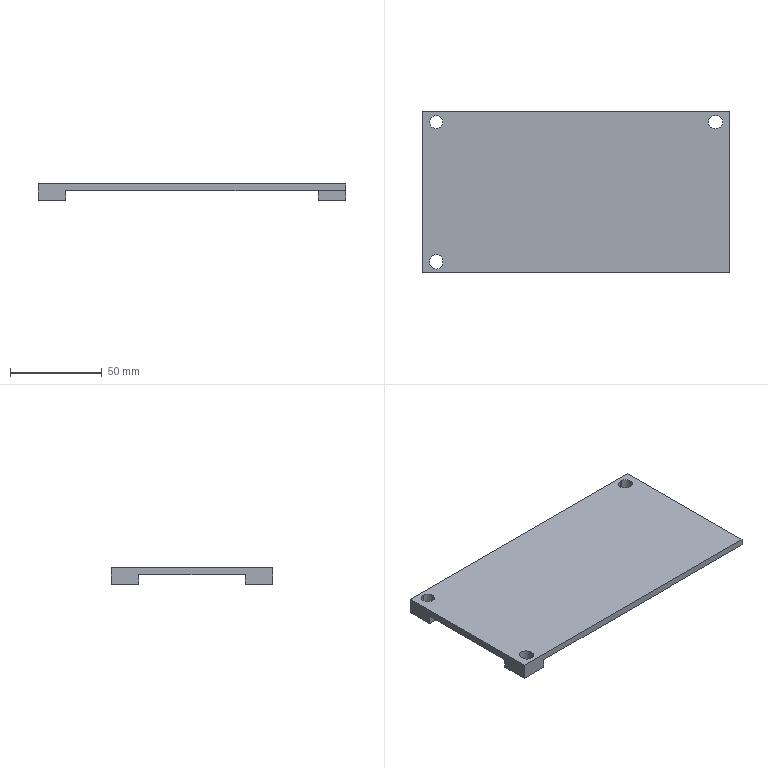NC program | NX | posted with a generic post | part box 168 x 88.2 x 8.8 mm
Lines 1 to 882 of 6992:
N10 G17 G21 G94 G90
(FLOOR_WALL , TOOL : D80)
N12 T19 M6
N14 G54
N16 G17 G0 G90 X-132. Y49.097 S5000 M3
N18 G43 Z30. H19
N20 Z3.
N22 G94 G1 Z0. F1200.
N24 X-129.
N26 X129.
N28 Y15.999
N30 X-129.
N32 Y-17.1
N34 X129.
N36 X132.
N38 Z3.
N40 G0 Z30.
N42 M5
(ADAPTIVE_MILLING , TOOL : D10)
N44 T15 M6
N46 G54
N48 G17 G0 G90 X-96.659 Y0.013 S9500 M3
N50 G43 Z30. H15
N52 Z-5.8
N54 G94 G1 Z-8.8 F1000.
N56 X-95.879 Y-0.266 F3000.
N58 X-95.09 Y-0.523
N60 G3 X-94.012 Y0.013 R1.017
N62 X-93.273 Y3.241 R9.097
N64 X-93.018 Y13.66 R133.26
N66 G1 X-93.014 Y16.36
N68 X-93.011 Y21.61
N70 Y46.135
N72 X-93.009 Y46.21
N74 X-93.003 Y46.36
N76 X-92.998 Y46.434
N78 G2 X-90.298 Y50.657 R5.929
N80 X-84.761 Y52.61 R12.858
N82 X-75.854 Y53.062 R69.734
N84 G1 X-74.504 Y53.071
N86 X-72.854 Y53.078
N88 X-70.529 Y53.083
N90 X-66.779 Y53.086
N92 X-54.779 Y53.087
N94 X85.996
N96 G2 X90.312 Y50.709 R5.649
N98 X92.436 Y45.322 R11.95
N100 X92.953 Y36.871 R57.592
N102 G1 X92.963 Y35.896
N104 X92.971 Y34.621
N106 X92.979 Y32.896
N108 X92.984 Y30.571
N110 X92.987 Y26.746
N112 X92.988 Y14.146
N114 Y-46.079
N116 X92.987 Y-46.154
N118 X92.983 Y-46.304
N120 X92.978 Y-46.379
N122 X92.972 Y-46.453
N124 G2 X90.314 Y-50.621 R5.924
N126 X84.564 Y-52.635 R12.965
N128 X75.431 Y-53.065 R74.74
N130 G1 X74.156 Y-53.073
N132 X72.431 Y-53.079
N134 X69.956 Y-53.084
N136 X65.606 Y-53.087
N138 X41.681
N140 X-35.494 Y-53.088
N142 X-36.019 Y-53.091
N144 X-37.069 Y-53.092
N146 X-37.594
N148 X-38.194 Y-53.094
N150 X-39.244
N152 X-40.144 Y-53.096
N154 X-41.344 Y-53.095
N156 X-42.019 Y-53.097
N158 X-43.219 Y-53.096
N160 X-43.819 Y-53.097
N162 X-44.944 Y-53.096
N164 X-45.319 Y-53.095
N166 X-45.994 Y-53.098
N168 X-47.269 Y-53.096
N170 X-47.944 Y-53.098
N172 X-49.144 Y-53.096
N174 X-49.969 Y-53.099
N176 X-50.719 Y-53.098
N178 X-51.769 Y-53.1
N180 X-52.444 Y-53.098
N182 X-53.569 Y-53.1
N184 X-54.169 Y-53.099
N186 X-55.294 Y-53.101
N188 X-55.669
N190 X-56.119 Y-53.1
N192 X-57.094 Y-53.101
N194 X-57.469
N196 X-57.994 Y-53.1
N198 X-59.194 Y-53.101
N200 X-59.869 Y-53.099
N202 X-61.069 Y-53.101
N204 X-61.894 Y-53.099
N206 X-63.094 Y-53.102
N208 X-63.619 Y-53.1
N210 X-65.194 Y-53.102
N212 X-65.719 Y-53.103
N214 X-66.244 Y-53.101
N216 X-67.444 Y-53.102
N218 X-68.344 Y-53.1
N220 X-69.244 Y-53.101
N222 X-69.994 Y-53.099
N224 X-71.119 Y-53.101
N226 X-71.869 Y-53.099
N228 X-72.769 Y-53.1
N230 X-73.519 Y-53.099
N232 X-74.419 Y-53.101
N234 X-75.019 Y-53.099
N236 X-76.219 Y-53.101
N238 X-76.894 Y-53.099
N240 X-77.944 Y-53.1
N242 X-78.619 Y-53.098
N244 X-79.594 Y-53.1
N246 X-80.194 Y-53.099
N248 X-81.244 Y-53.101
N250 X-81.619
N252 X-82.144 Y-53.1
N254 G2 X-86.642 Y-53.049 R55.93
N256 X-90.766 Y-50.059 R6.199
N258 X-92.602 Y-44.164 R14.147
N260 X-92.973 Y-34.276 R94.705
N262 G1 X-92.98 Y-32.626
N264 X-92.984 Y-30.151
N266 X-92.987 Y-25.876
N268 X-92.988 Y-6.526
N270 Y-3.826
N272 X-92.985 Y-3.601
N274 G2 X-92.416 Y2.144 R99.297
N276 G3 X-92.035 Y14.659 R147.053
N278 G1 X-92.029 Y16.834
N280 X-92.025 Y19.984
N282 X-92.023 Y26.209
N284 X-92.022 Y43.009
N286 X-92.02 Y43.159
N288 X-92.019 Y43.234
N290 G2 X-88.333 Y49.422 R7.66
N292 X-81.987 Y51.558 R15.465
N294 X-72.781 Y52.041 R76.235
N296 G1 X-71.581 Y52.051
N298 X-70.156 Y52.06
N300 X-68.281 Y52.067
N302 X-65.731 Y52.072
N304 X-61.381 Y52.075
N306 X-45.106 Y52.076
N308 X82.919
N310 X83.069 Y52.074
N312 X83.219 Y52.07
N314 X83.369 Y52.063
N316 X83.519 Y52.053
N318 G2 X89.452 Y48.198 R7.743
N320 X91.482 Y41.892 R15.917
N322 X91.95 Y31.859 R85.406
N324 G1 X91.96 Y30.434
N326 X91.967 Y28.634
N328 X91.972 Y26.159
N330 X91.975 Y22.109
N332 X91.977 Y9.884
N334 Y-31.216
N336 G2 X91.95 Y-43.74 R466.461
N338 X88.059 Y-49.573 R7.789
N340 X81.598 Y-51.609 R16.275
N342 X72.238 Y-52.046 R85.328
N344 G1 X70.963 Y-52.056
N346 X69.388 Y-52.063
N348 X67.288 Y-52.069
N350 X64.138 Y-52.074
N352 X57.838 Y-52.076
N354 X-32.462
N356 X-33.287 Y-52.082
N358 X-34.412
N360 X-35.237 Y-52.086
N362 X-36.287 Y-52.087
N364 X-36.662
N366 X-37.337 Y-52.09
N368 X-38.312
N370 X-39.212 Y-52.093
N372 X-40.337 Y-52.092
N374 X-41.012 Y-52.094
N376 X-41.912 Y-52.093
N378 X-42.362 Y-52.092
N380 X-43.187 Y-52.095
N382 X-44.312 Y-52.093
N384 X-44.987 Y-52.095
N386 X-46.187 Y-52.094
N388 X-46.562
N390 X-47.162 Y-52.096
N392 X-48.362 Y-52.095
N394 X-49.112 Y-52.097
N396 X-50.162 Y-52.096
N398 X-50.762 Y-52.098
N400 X-52.037 Y-52.097
N402 X-52.637 Y-52.099
N404 X-53.687 Y-52.098
N406 X-54.512 Y-52.101
N408 X-55.262 Y-52.1
N410 X-56.312 Y-52.101
N412 X-57.212 Y-52.1
N414 X-58.112 Y-52.101
N416 X-58.487 Y-52.102
N418 X-59.236 Y-52.099
N420 X-60.361 Y-52.102
N422 X-61.036 Y-52.101
N424 X-62.086 Y-52.102
N426 X-62.761 Y-52.104
N428 X-63.361 Y-52.103
N430 X-64.936
N432 X-65.686 Y-52.105
N434 X-66.211 Y-52.103
N436 X-67.261 Y-52.104
N438 X-68.161 Y-52.106
N440 X-68.761 Y-52.103
N442 X-69.886 Y-52.104
N444 G2 X-83.536 Y-52.075 R830.143
N446 X-89.419 Y-48.263 R7.764
N448 X-91.483 Y-41.891 R15.898
N450 X-91.949 Y-32.008 R84.57
N452 G1 X-91.959 Y-30.658
N454 X-91.966 Y-28.933
N456 X-91.971 Y-26.608
N458 X-91.975 Y-22.933
N460 X-91.976 Y-13.933
N462 Y-6.133
N464 G2 X-91.522 Y0.9 R88.839
N466 G3 X-91.046 Y17.013 R201.872
N468 G1 X-91.04 Y19.563
N470 X-91.036 Y23.388
N472 X-91.034 Y31.413
N474 X-91.033 Y40.038
N476 X-91.031 Y40.413
N478 X-91.027 Y40.638
N480 G2 X-87.928 Y47.368 R8.693
N482 X-85.91 Y48.894 R5.21
N484 X-78.589 Y50.684 R21.893
N486 X-67.498 Y51.046 R132.801
N488 G1 X-65.623 Y51.054
N490 X-63.148 Y51.059
N492 X-59.248 Y51.063
N494 X-49.798 Y51.064
N496 X80.327 Y51.065
N498 X80.627 Y51.06
N500 G2 X87.148 Y48.12 R8.608
N502 X88.694 Y46.211 R5.049
N504 X90.561 Y38.912 R21.152
N506 X90.944 Y28.123 R122.229
N508 G1 X90.952 Y26.473
N510 X90.958 Y24.298
N512 X90.962 Y21.073
N514 X90.965 Y14.923
N516 X90.966 Y-28.202
N518 X90.969 Y-28.802
N520 G2 X90.955 Y-41.251 R725.465
N522 X88.012 Y-47.259 R8.599
N524 X86.111 Y-48.794 R5.052
N526 X78.737 Y-50.667 R21.271
N528 X67.723 Y-51.045 R126.708
N530 G1 X65.923 Y-51.053
N532 X63.523 Y-51.059
N534 X59.998 Y-51.062
N536 X52.273 Y-51.064
N538 X-29.477 Y-51.065
N540 X-30.302 Y-51.07
N542 X-31.352 Y-51.072
N544 X-31.727
N546 X-32.252 Y-51.075
N548 X-33.602 Y-51.078
N550 X-34.127
N552 X-34.802 Y-51.082
N554 X-35.552 Y-51.083
N556 X-35.927
N558 X-36.602 Y-51.086
N560 X-37.577 Y-51.087
N562 X-37.952
N564 X-38.402 Y-51.089
N566 X-39.452
N568 X-39.827
N570 X-40.427 Y-51.092
N572 X-41.477 Y-51.091
N574 X-42.227 Y-51.093
N576 X-43.502 Y-51.091
N578 X-44.177 Y-51.093
N580 X-45.302 Y-51.092
N582 X-45.677
N584 X-46.277 Y-51.094
N586 X-47.402
N588 X-48.077 Y-51.096
N590 X-49.202 Y-51.094
N592 X-50.027 Y-51.097
N594 X-51.002 Y-51.096
N596 X-51.752 Y-51.098
N598 X-52.877 Y-51.097
N600 X-53.552 Y-51.099
N602 X-54.677 Y-51.098
N604 X-55.052
N606 X-55.652 Y-51.099
N608 X-56.552
N610 X-56.927 Y-51.098
N612 X-57.677 Y-51.101
N614 X-58.502 Y-51.1
N616 X-59.402 Y-51.102
N618 X-59.777 Y-51.103
N620 X-60.527 Y-51.102
N622 X-61.652 Y-51.104
N624 X-62.327 Y-51.103
N626 X-63.227 Y-51.104
N628 X-63.977 Y-51.102
N630 X-64.652 Y-51.104
N632 X-65.102 Y-51.105
N634 X-66.227 Y-51.102
N636 X-67.127 Y-51.105
N638 X-68.102 Y-51.102
N640 X-68.927 Y-51.104
N642 X-69.827 Y-51.102
N644 X-70.952 Y-51.104
N646 X-71.777 Y-51.102
N648 X-72.677 Y-51.103
N650 X-73.652 Y-51.101
N652 X-74.777 Y-51.103
N654 X-75.452 Y-51.102
N656 X-76.577 Y-51.103
N658 X-76.952
N660 X-77.627 Y-51.101
N662 G2 X-82.046 Y-50.974 R32.659
N664 X-87.199 Y-48.081 R8.637
N666 X-88.66 Y-46.278 R5.013
N668 X-90.56 Y-38.912 R21.138
N670 X-90.947 Y-27.447 R128.239
N672 G1 X-90.955 Y-25.572
N674 X-90.96 Y-23.097
N676 X-90.964 Y-19.197
N678 X-90.965 Y-9.447
N680 Y-7.872
N682 X-90.96 Y-7.197
N684 G2 X-90.373 Y3.135 R256.242
N686 G3 X-90.05 Y22.18 R382.724
N688 G2 X-90.009 Y39.054 R953.587
N690 X-89.166 Y42.842 R11.59
N692 X-88.948 Y45.497 R12.88
N694 X-87.915 Y47.385 R5.352
N696 G1 X-87.759 Y47.591
N698 X-87.586 Y47.784
N700 X-86.63 Y48.518
N702 X-86.511 Y48.587
N704 G2 X-83.515 Y49.254 R6.135
N706 X-66.215 Y50.03 R172.99
N708 G1 X-64.415 Y50.039
N710 X-62.09 Y50.045
N712 X-58.79 Y50.05
N714 X-52.94 Y50.052
N716 X10.735 Y50.053
N718 X78.01
N720 G2 X82.636 Y49.258 R12.734
N722 X85.397 Y49.048 R12.239
N724 X87.166 Y48.107 R5.201
N726 G1 X86.847 Y48.358
N728 X86.511 Y48.587
N730 G3 X83.965 Y49.25 R6.124
N732 G1 X82.711
N734 G3 X67.864 Y49.446 R300.003
N736 G1 X-61.661 Y49.447
N738 X-61.961 Y49.445
N740 X-62.111
N742 X-62.636 Y49.442
N744 X-62.786
N746 G3 X-74.872 Y49.25 R373.405
N748 G1 X-83.647
N750 X82.403
N752 G2 X85.397 Y49.048 R12.741
N754 X88.487 Y46.611 R5.458
N756 X89.15 Y43.69 R6.026
N758 X89.94 Y24.29 R189.119
N760 G1 X89.947 Y21.89
N762 X89.951 Y18.44
N764 X89.953 Y11.915
N766 X89.954 Y-25.21
N768 X89.958 Y-25.81
N770 X89.96 Y-26.935
N772 G2 X89.941 Y-39.309 R466.914
N774 X89.165 Y-42.732 R11.596
N776 X88.948 Y-45.497 R13.211
N778 X88.007 Y-47.266 R5.201
N780 G1 X88.258 Y-46.947
N782 X88.487 Y-46.611
N784 G3 X89.15 Y-44.065 R6.124
N786 G1 Y-42.853
N788 G3 X89.358 Y-28.833 R232.088
N790 G1 X89.354 Y-26.883
N792 X89.353 Y-25.308
N794 X89.352 Y-24.483
N796 X89.355 Y-22.683
N798 X89.353 Y-20.658
N800 Y-20.208
N802 X89.355 Y-18.483
N804 X89.354 Y-16.308
N806 X89.353 Y-15.708
N808 Y-14.883
N810 X89.354 Y-13.008
N812 X89.355 Y-12.408
N814 X89.353 Y-10.158
N816 Y-9.783
N818 X89.354 Y-7.308
N820 X89.355 Y-6.858
N822 X89.353 Y-4.608
N824 Y-4.233
N826 X89.354 Y-2.208
N828 X89.355 Y-1.833
N830 X89.353 Y0.192
N832 Y0.642
N834 X89.355 Y2.367
N836 X89.354 Y3.942
N838 X89.352 Y4.617
N840 X89.353 Y5.142
N842 X89.354 Y7.017
N844 X89.355 Y7.617
N846 X89.353 Y9.867
N848 X89.352 Y10.392
N850 X89.354 Y12.192
N852 X89.352 Y14.217
N854 X89.351 Y14.742
N856 X89.353 Y16.542
N858 X89.352 Y17.067
N860 Y17.292
N862 X89.351 Y17.592
N864 X89.352 Y17.817
N866 X89.35 Y18.492
N868 X89.351 Y18.717
N870 X89.349 Y19.092
N872 Y19.242
N874 X89.348 Y19.542
N876 X89.349 Y19.692
N878 X89.347 Y20.142
N880 Y20.292
N882 X89.345 Y20.967
N884 Y21.117
N886 X89.327 Y26.292
N888 X89.312 Y27.942
N890 G3 X89.15 Y34.956 R557.163
N892 G1 Y43.731
N894 Y-42.519
N896 G2 X88.948 Y-45.497 R12.654
N898 X86.511 Y-48.587 R5.458
N900 X83.59 Y-49.25 R6.026
N902 X65.39 Y-50.035 R182.187
N904 G1 X63.365 Y-50.042
N906 X60.665 Y-50.048
N908 X56.54 Y-50.051
N910 X46.64 Y-50.053
N912 X-8.185
N914 X-9.385 Y-50.059
N916 X-10.135
N918 X-10.96 Y-50.061
N920 X-12.01 Y-50.06
N922 X-12.76 Y-50.063
N924 X-13.735 Y-50.061
N926 X-14.335 Y-50.063
N928 X-15.385 Y-50.062
N930 X-15.76
N932 X-16.21 Y-50.063
N934 X-17.41 Y-50.062
N936 X-18.01 Y-50.064
N938 X-18.985 Y-50.062
N940 X-19.36
N942 X-19.885 Y-50.064
N944 X-20.935 Y-50.062
N946 X-21.31
N948 X-21.76 Y-50.064
N950 X-22.885 Y-50.062
N952 X-23.56 Y-50.064
N954 X-24.76 Y-50.062
N956 X-25.585 Y-50.065
N958 X-26.56 Y-50.063
N960 X-27.76 Y-50.067
N962 X-28.66 Y-50.066
N964 X-29.935 Y-50.072
N966 X-30.46
N968 X-32.11 Y-50.077
N970 X-32.71 Y-50.08
N972 X-33.235
N974 X-34.66 Y-50.084
N976 X-35.41 Y-50.087
N978 X-36.685 Y-50.085
N980 X-37.21 Y-50.086
N982 X-39.16 Y-50.087
N984 X-40.51 Y-50.086
N986 X-41.26 Y-50.089
N988 X-42.31 Y-50.088
N990 X-42.685
N992 X-43.36 Y-50.09
N994 X-44.56
N996 X-45.235 Y-50.093
N998 X-45.985 Y-50.092
N1000 X-46.435 Y-50.091
N1002 X-47.26 Y-50.094
N1004 X-48.235 Y-50.093
N1006 X-49.209 Y-50.097
N1008 X-50.109 Y-50.095
N1010 X-51.009 Y-50.098
N1012 X-52.209 Y-50.095
N1014 X-53.034 Y-50.098
N1016 X-53.934 Y-50.097
N1018 X-54.909 Y-50.099
N1020 X-55.734 Y-50.098
N1022 X-56.859 Y-50.101
N1024 X-57.609 Y-50.1
N1026 X-58.734 Y-50.103
N1028 X-59.634 Y-50.101
N1030 X-60.534 Y-50.104
N1032 X-61.284 Y-50.102
N1034 X-62.259 Y-50.104
N1036 X-62.634 Y-50.105
N1038 X-63.309 Y-50.103
N1040 X-64.359 Y-50.105
N1042 X-64.734
N1044 X-65.409 Y-50.103
N1046 X-66.384 Y-50.104
N1048 X-67.209 Y-50.102
N1050 X-68.109 Y-50.104
N1052 X-68.934 Y-50.103
N1054 X-69.984 Y-50.104
N1056 X-70.809 Y-50.102
N1058 X-71.934 Y-50.104
N1060 X-72.834 Y-50.102
N1062 X-73.659 Y-50.104
N1064 X-74.784 Y-50.101
N1066 G2 X-80.029 Y-49.977 R46.83
N1068 X-82.702 Y-49.26 R14.403
N1070 X-85.397 Y-49.048 R12.192
N1072 X-87.225 Y-48.061 R5.27
N1074 G1 X-86.877 Y-48.336
N1076 X-86.511 Y-48.587
N1078 G3 X-83.965 Y-49.25 R6.124
N1080 G1 X-82.786
N1082 G3 X-70.641 Y-49.497 R193.895
N1084 G1 X-61.791 Y-49.5
N1086 X-52.941 Y-49.499
N1088 X-44.091 Y-49.494
N1090 X-35.241 Y-49.485
N1092 X-31.941 Y-49.48
N1094 X-31.491 Y-49.477
N1096 X-31.191 Y-49.476
N1098 X-29.316 Y-49.474
N1100 X-29.091 Y-49.472
N1102 X-20.541 Y-49.46
N1104 X-20.166 Y-49.461
N1106 X-19.341 Y-49.459
N1108 X-19.041 Y-49.461
N1110 X-18.666 Y-49.46
N1112 X-18.516 Y-49.461
N1114 X-17.541 Y-49.459
N1116 X-17.316 Y-49.46
N1118 X-17.016
N1120 X-16.866
N1122 X-15.816 Y-49.459
N1124 X-15.516 Y-49.46
N1126 X-15.216
N1128 X-15.066
N1130 X-14.316 Y-49.459
N1132 X-13.866 Y-49.46
N1134 X-13.116
N1136 X-11.991 Y-49.458
N1138 X-11.766 Y-49.459
N1140 X-10.491 Y-49.455
N1142 X-10.116
N1144 X-8.392
N1146 X-8.017
N1148 X-5.767
N1150 X-3.742
N1152 X-3.442
N1154 X-3.292
N1156 X-2.992
N1158 X-2.842
N1160 X-2.542
N1162 X-2.392
N1164 X-2.092
N1166 X-1.942
N1168 X-1.642
N1170 X-1.492
N1172 X-1.192
N1174 X-1.042
N1176 X-0.742
N1178 X-0.592
N1180 X-0.292
N1182 X-0.142
N1184 X0.158
N1186 X0.308
N1188 X0.608
N1190 X0.758
N1192 X1.058
N1194 X1.208
N1196 X1.508
N1198 X1.658
N1200 X1.958
N1202 X2.108
N1204 X2.408
N1206 X2.558
N1208 X2.858
N1210 X3.008
N1212 X3.308
N1214 X3.458
N1216 X3.758
N1218 X3.908
N1220 X4.208
N1222 X4.358
N1224 X4.658
N1226 X4.808
N1228 X5.108
N1230 X5.258
N1232 X5.558
N1234 X5.708
N1236 X6.008
N1238 X6.158
N1240 X6.458
N1242 X6.608
N1244 X6.908
N1246 X7.058
N1248 X7.358
N1250 X7.508
N1252 X7.808
N1254 X7.958
N1256 X8.258
N1258 X8.408
N1260 X8.708
N1262 X8.858
N1264 X9.158
N1266 X9.308
N1268 X9.608
N1270 X9.758
N1272 X10.058
N1274 X10.208
N1276 X10.508 Y-49.456
N1278 X10.658 Y-49.455
N1280 X10.958 Y-49.456
N1282 X11.108 Y-49.455
N1284 X11.408 Y-49.456
N1286 X11.558 Y-49.455
N1288 X11.858 Y-49.456
N1290 X12.008 Y-49.455
N1292 X12.308 Y-49.456
N1294 X12.458 Y-49.455
N1296 X12.758 Y-49.456
N1298 X12.908 Y-49.455
N1300 X13.208 Y-49.456
N1302 X13.358 Y-49.455
N1304 X13.658 Y-49.456
N1306 X13.808 Y-49.455
N1308 X14.108 Y-49.456
N1310 X14.258 Y-49.455
N1312 X14.558 Y-49.456
N1314 X14.708 Y-49.455
N1316 X15.008 Y-49.456
N1318 X15.158 Y-49.455
N1320 X15.458 Y-49.456
N1322 X15.608 Y-49.455
N1324 X15.908 Y-49.456
N1326 X16.058 Y-49.455
N1328 X16.358 Y-49.456
N1330 X16.508 Y-49.455
N1332 X16.808 Y-49.456
N1334 X16.958 Y-49.455
N1336 X17.258 Y-49.456
N1338 X17.408 Y-49.455
N1340 X17.708 Y-49.456
N1342 X17.858 Y-49.455
N1344 X18.158 Y-49.456
N1346 X18.308 Y-49.455
N1348 X18.608 Y-49.456
N1350 X18.758 Y-49.455
N1352 X19.058 Y-49.456
N1354 X19.208 Y-49.455
N1356 X19.508 Y-49.456
N1358 X19.658 Y-49.455
N1360 X19.958 Y-49.456
N1362 X20.108 Y-49.455
N1364 X20.408 Y-49.456
N1366 X20.558 Y-49.455
N1368 X20.858 Y-49.456
N1370 X21.008 Y-49.455
N1372 X21.308 Y-49.456
N1374 X21.458 Y-49.455
N1376 X21.758 Y-49.456
N1378 X21.908 Y-49.455
N1380 X22.208 Y-49.456
N1382 X22.358 Y-49.455
N1384 X22.658 Y-49.456
N1386 X22.808 Y-49.455
N1388 X23.108 Y-49.456
N1390 X23.258 Y-49.455
N1392 X23.558 Y-49.456
N1394 X23.708 Y-49.455
N1396 X24.008 Y-49.456
N1398 X24.158 Y-49.455
N1400 X24.458 Y-49.456
N1402 X24.608 Y-49.455
N1404 X24.908 Y-49.456
N1406 X25.058 Y-49.455
N1408 X25.358 Y-49.456
N1410 X25.508 Y-49.455
N1412 X25.808 Y-49.456
N1414 X25.958 Y-49.455
N1416 X26.258 Y-49.456
N1418 X26.408 Y-49.455
N1420 X26.708 Y-49.456
N1422 X26.858 Y-49.455
N1424 X27.158 Y-49.456
N1426 X27.308 Y-49.455
N1428 X27.608 Y-49.456
N1430 X27.758 Y-49.455
N1432 X28.058 Y-49.456
N1434 X28.208 Y-49.455
N1436 X28.508 Y-49.456
N1438 X28.658 Y-49.455
N1440 X28.958 Y-49.456
N1442 X29.108 Y-49.455
N1444 X29.408 Y-49.456
N1446 X29.558 Y-49.455
N1448 X29.858 Y-49.456
N1450 X30.008 Y-49.455
N1452 X30.308 Y-49.456
N1454 X30.458 Y-49.455
N1456 X30.758 Y-49.456
N1458 X30.908 Y-49.455
N1460 X31.208 Y-49.456
N1462 X31.733 Y-49.455
N1464 X32.033
N1466 X32.183
N1468 X32.483
N1470 X32.633
N1472 X32.933
N1474 X33.083
N1476 X33.383
N1478 X33.533
N1480 X33.833
N1482 X33.983
N1484 X34.283
N1486 X34.433
N1488 X34.733
N1490 X34.883
N1492 X35.183
N1494 X35.333
N1496 X35.633
N1498 X35.783
N1500 X36.083
N1502 X36.233
N1504 X36.533
N1506 X36.683
N1508 X36.983
N1510 X37.133
N1512 X37.433
N1514 X37.583
N1516 X37.883
N1518 X38.033
N1520 X38.333
N1522 X38.483
N1524 X38.783
N1526 X38.933
N1528 X39.233
N1530 X39.383
N1532 X39.683
N1534 X39.833
N1536 X40.133
N1538 X40.283
N1540 X40.583
N1542 X40.733
N1544 X41.033
N1546 X41.183
N1548 X41.483
N1550 X41.633
N1552 X41.933
N1554 X42.083
N1556 X42.383
N1558 X42.533
N1560 X42.833
N1562 X42.983
N1564 X43.283
N1566 X43.433
N1568 X43.733
N1570 X43.883
N1572 X44.183
N1574 X44.333
N1576 X44.633
N1578 X45.158
N1580 X45.458
N1582 X45.608
N1584 X45.908
N1586 X46.058
N1588 X46.358
N1590 X46.508
N1592 X46.808
N1594 X47.333
N1596 X47.633
N1598 X47.783
N1600 X48.083
N1602 X48.233
N1604 X48.533
N1606 X49.058
N1608 X49.358
N1610 X49.883 Y-49.454
N1612 X50.183 Y-49.455
N1614 X50.708 Y-49.454
N1616 X51.008 Y-49.455
N1618 X51.533 Y-49.454
N1620 X51.833 Y-49.455
N1622 X52.058 Y-49.454
N1624 X52.358
N1626 X54.608
N1628 X54.833 Y-49.453
N1630 X55.433
N1632 X55.658 Y-49.452
N1634 X55.883 Y-49.453
N1636 X56.108 Y-49.452
N1638 G3 X74.875 Y-49.25 R527.988
N1640 G1 X83.65
N1642 X-82.55
N1644 G2 X-85.397 Y-49.048 R11.969
N1646 X-88.487 Y-46.611 R5.458
N1648 X-89.157 Y-43.54 R6.255
N1650 X-89.936 Y-25.265 R176.655
N1652 X-89.893 Y-6.141 R804.849
N1654 G3 X-89.209 Y7.716 R879.487
N1656 G1 X-89.184 Y8.766
N1658 X-89.159 Y9.966
N1660 X-89.15 Y10.469
N1662 Y43.019
N1664 G3 X-90.866 Y43.717 R1.001
N1666 X-91.191 Y43.089 Z-8.764 R1.655
N1668 G1 X-91.639 Y41.883 Z-8.7
N1670 X-92.304 Y40.071
N1672 X-92.332 Y39.837
N1674 Y13.651
N1676 G3 X-91.884 Y12.817 R1.014
N1678 G1 X-91.6 Y12.628
N1680 X-89.932 Y11.524 Z-8.8
N1682 X-89.469 Y11.201
N1684 G2 X-89.15 Y10.469 R1.026
N1686 X-89.195 Y-3.256 R590.313
N1688 G3 X-89.344 Y-18.104 R389.695
N1690 X-89.15 Y-35.018 R449.919
N1692 G1 Y-43.718
N1694 Y-1.643
N1696 G3 X-89.998 Y-0.646 R1.016
N1698 G1 X-91.55 Y-0.393
N1700 Z-5.8
N1702 G0 Z30.
N1704 M5
(ZLEVEL_PROFILE_COPY , TOOL : D10JING)
N1706 T14 M6
N1708 G54
N1710 G17 G0 G90 X-89. Y23.357 S9500 M3
N1712 G43 Z30. H14
N1714 Z-7.3
N1716 G94 G1 Y44.649 Z-8.416 F1000.
N1718 X-88.672 Y45.964 Z-8.487
N1720 X-88.004 Y47.145 Z-8.558
N1722 X-87.045 Y48.104 Z-8.629
N1724 X-85.864 Y48.772 Z-8.7
N1726 X-84.549 Y49.1 Z-8.771
N1728 X-84. Z-8.8
N1730 X84. F1500.
N1732 G2 X89. Y44.1 R5.
N1734 G1 Y-44.1
N1736 G2 X84. Y-49.1 R5.
N1738 G1 X-84.
N1740 G2 X-89. Y-44.1 R5.
N1742 G1 Y44.1
N1744 G2 X-84. Y49.1 R5.
N1746 G1 Z-7.3
N1748 G0 Z30.
N1750 M5